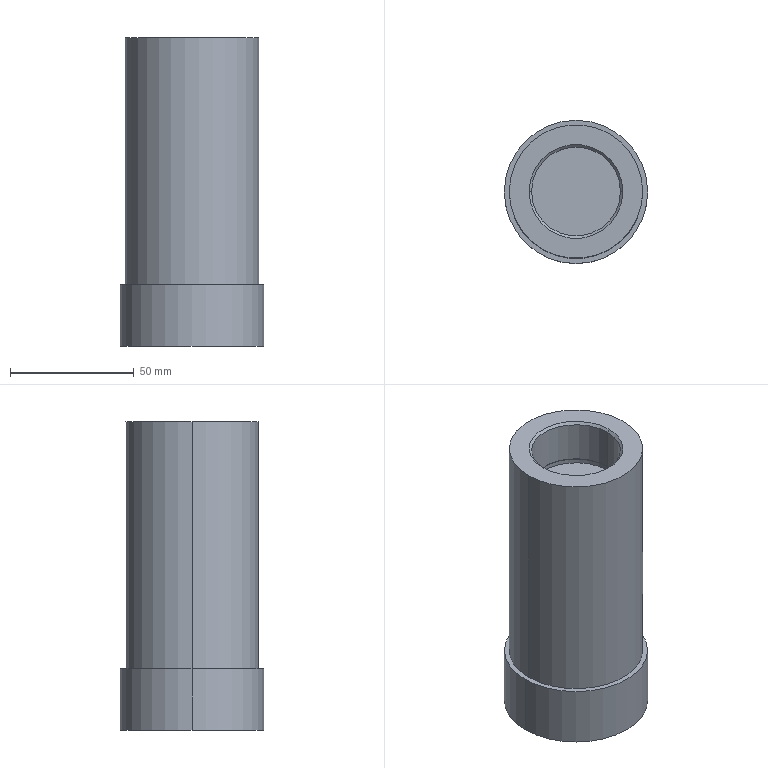Part | SolidWorks | features ICE 5, Chamfer 2, Extrusion 1 | 1 solid | 23 faces | box 58 x 58 x 125 mm | volume 229241 mm3 | cylinder 12 | plane 7 | cone 4 | commonest cylinder face diameters 36 x2 36.5 x2 48 x2 48.2 x2 54 x2 58 x2
STEP:
#1=CARTESIAN_POINT('',(-18.,0.,124.));
#2=VERTEX_POINT('',#1);
#3=CARTESIAN_POINT('',(18.,0.,124.));
#4=VERTEX_POINT('',#3);
#5=CARTESIAN_POINT('',(0.,0.,124.));
#6=DIRECTION('',(0.,0.,1.));
#7=DIRECTION('',(1.,0.,0.));
#8=AXIS2_PLACEMENT_3D('',#5,#6,#7);
#9=CIRCLE('',#8,18.);
#10=EDGE_CURVE('',#2,#4,#9,.T.);
#11=ORIENTED_EDGE('',*,*,#10,.F.);
#12=CARTESIAN_POINT('',(-19.,0.,125.));
#13=VERTEX_POINT('',#12);
#14=CARTESIAN_POINT('',(-18.,0.,124.));
#15=DIRECTION('',(-0.7071,0.,0.7071));
#16=VECTOR('',#15,1000.);
#17=LINE('',#14,#16);
#18=EDGE_CURVE('',#2,#13,#17,.T.);
#19=ORIENTED_EDGE('',*,*,#18,.T.);
#20=CARTESIAN_POINT('',(19.,0.,125.));
#21=VERTEX_POINT('',#20);
#22=CARTESIAN_POINT('',(0.,0.,125.));
#23=DIRECTION('',(0.,0.,-1.));
#24=DIRECTION('',(1.,0.,0.));
#25=AXIS2_PLACEMENT_3D('',#22,#23,#24);
#26=CIRCLE('',#25,19.);
#27=EDGE_CURVE('',#21,#13,#26,.T.);
#28=ORIENTED_EDGE('',*,*,#27,.F.);
#29=CARTESIAN_POINT('',(18.,0.,124.));
#30=DIRECTION('',(0.7071,0.,0.7071));
#31=VECTOR('',#30,1000.);
#32=LINE('',#29,#31);
#33=EDGE_CURVE('',#4,#21,#32,.T.);
#34=ORIENTED_EDGE('',*,*,#33,.F.);
#35=EDGE_LOOP('',(#11,#19,#28,#34));
#36=FACE_OUTER_BOUND('',#35,.T.);
#37=CARTESIAN_POINT('',(0.,0.,124.));
#38=DIRECTION('',(0.,0.,1.));
#39=DIRECTION('',(1.,0.,0.));
#40=AXIS2_PLACEMENT_3D('',#37,#38,#39);
#41=CONICAL_SURFACE('',#40,18.,0.7854);
#42=ADVANCED_FACE('',(#36),#41,.F.);
#43=CARTESIAN_POINT('',(-18.25,0.,105.));
#44=VERTEX_POINT('',#43);
#45=CARTESIAN_POINT('',(18.25,0.,105.));
#46=VERTEX_POINT('',#45);
#47=CARTESIAN_POINT('',(0.,0.,105.));
#48=DIRECTION('',(0.,0.,1.));
#49=DIRECTION('',(1.,0.,0.));
#50=AXIS2_PLACEMENT_3D('',#47,#48,#49);
#51=CIRCLE('',#50,18.25);
#52=EDGE_CURVE('',#44,#46,#51,.T.);
#53=ORIENTED_EDGE('',*,*,#52,.F.);
#54=CARTESIAN_POINT('',(-18.25,0.,107.));
#55=VERTEX_POINT('',#54);
#56=CARTESIAN_POINT('',(-18.25,0.,105.));
#57=DIRECTION('',(0.,0.,1.));
#58=VECTOR('',#57,1000.);
#59=LINE('',#56,#58);
#60=EDGE_CURVE('',#44,#55,#59,.T.);
#61=ORIENTED_EDGE('',*,*,#60,.T.);
#62=CARTESIAN_POINT('',(18.25,0.,107.));
#63=VERTEX_POINT('',#62);
#64=CARTESIAN_POINT('',(0.,0.,107.));
#65=DIRECTION('',(0.,0.,1.));
#66=DIRECTION('',(1.,0.,0.));
#67=AXIS2_PLACEMENT_3D('',#64,#65,#66);
#68=CIRCLE('',#67,18.25);
#69=EDGE_CURVE('',#55,#63,#68,.T.);
#70=ORIENTED_EDGE('',*,*,#69,.T.);
#71=CARTESIAN_POINT('',(18.25,0.,105.));
#72=DIRECTION('',(0.,0.,1.));
#73=VECTOR('',#72,1000.);
#74=LINE('',#71,#73);
#75=EDGE_CURVE('',#46,#63,#74,.T.);
#76=ORIENTED_EDGE('',*,*,#75,.F.);
#77=EDGE_LOOP('',(#53,#61,#70,#76));
#78=FACE_OUTER_BOUND('',#77,.T.);
#79=CARTESIAN_POINT('',(0.,0.,105.));
#80=DIRECTION('',(0.,0.,1.));
#81=DIRECTION('',(1.,0.,0.));
#82=AXIS2_PLACEMENT_3D('',#79,#80,#81);
#83=CYLINDRICAL_SURFACE('',#82,18.25);
#84=ADVANCED_FACE('',(#78),#83,.F.);
#85=CARTESIAN_POINT('',(-18.,0.,107.));
#86=VERTEX_POINT('',#85);
#87=CARTESIAN_POINT('',(18.,0.,107.));
#88=VERTEX_POINT('',#87);
#89=CARTESIAN_POINT('',(0.,0.,107.));
#90=DIRECTION('',(0.,0.,1.));
#91=DIRECTION('',(1.,0.,0.));
#92=AXIS2_PLACEMENT_3D('',#89,#90,#91);
#93=CIRCLE('',#92,18.);
#94=EDGE_CURVE('',#86,#88,#93,.T.);
#95=ORIENTED_EDGE('',*,*,#94,.F.);
#96=CARTESIAN_POINT('',(-18.,0.,107.));
#97=DIRECTION('',(0.,0.,1.));
#98=VECTOR('',#97,1000.);
#99=LINE('',#96,#98);
#100=EDGE_CURVE('',#86,#2,#99,.T.);
#101=ORIENTED_EDGE('',*,*,#100,.T.);
#102=ORIENTED_EDGE('',*,*,#10,.T.);
#103=CARTESIAN_POINT('',(18.,0.,107.));
#104=DIRECTION('',(0.,0.,1.));
#105=VECTOR('',#104,1000.);
#106=LINE('',#103,#105);
#107=EDGE_CURVE('',#88,#4,#106,.T.);
#108=ORIENTED_EDGE('',*,*,#107,.F.);
#109=EDGE_LOOP('',(#95,#101,#102,#108));
#110=FACE_OUTER_BOUND('',#109,.T.);
#111=CARTESIAN_POINT('',(0.,0.,107.));
#112=DIRECTION('',(0.,0.,1.));
#113=DIRECTION('',(1.,0.,0.));
#114=AXIS2_PLACEMENT_3D('',#111,#112,#113);
#115=CYLINDRICAL_SURFACE('',#114,18.);
#116=ADVANCED_FACE('',(#110),#115,.F.);
#117=CARTESIAN_POINT('',(24.,0.,1.));
#118=VERTEX_POINT('',#117);
#119=CARTESIAN_POINT('',(-24.,0.,1.));
#120=VERTEX_POINT('',#119);
#121=CARTESIAN_POINT('',(0.,0.,1.));
#122=DIRECTION('',(0.,0.,-1.));
#123=DIRECTION('',(1.,0.,0.));
#124=AXIS2_PLACEMENT_3D('',#121,#122,#123);
#125=CIRCLE('',#124,24.);
#126=EDGE_CURVE('',#118,#120,#125,.T.);
#127=ORIENTED_EDGE('',*,*,#126,.F.);
#128=CARTESIAN_POINT('',(25.,0.,0.));
#129=VERTEX_POINT('',#128);
#130=CARTESIAN_POINT('',(24.,0.,1.));
#131=DIRECTION('',(0.7071,0.,-0.7071));
#132=VECTOR('',#131,1000.);
#133=LINE('',#130,#132);
#134=EDGE_CURVE('',#118,#129,#133,.T.);
#135=ORIENTED_EDGE('',*,*,#134,.T.);
#136=CARTESIAN_POINT('',(-25.,0.,0.));
#137=VERTEX_POINT('',#136);
#138=CARTESIAN_POINT('',(0.,0.,0.));
#139=DIRECTION('',(0.,0.,1.));
#140=DIRECTION('',(1.,0.,0.));
#141=AXIS2_PLACEMENT_3D('',#138,#139,#140);
#142=CIRCLE('',#141,25.);
#143=EDGE_CURVE('',#137,#129,#142,.T.);
#144=ORIENTED_EDGE('',*,*,#143,.F.);
#145=CARTESIAN_POINT('',(-24.,0.,1.));
#146=DIRECTION('',(-0.7071,0.,-0.7071));
#147=VECTOR('',#146,1000.);
#148=LINE('',#145,#147);
#149=EDGE_CURVE('',#120,#137,#148,.T.);
#150=ORIENTED_EDGE('',*,*,#149,.F.);
#151=EDGE_LOOP('',(#127,#135,#144,#150));
#152=FACE_OUTER_BOUND('',#151,.T.);
#153=CARTESIAN_POINT('',(0.,0.,1.));
#154=DIRECTION('',(0.,0.,-1.));
#155=DIRECTION('',(-1.,0.,0.));
#156=AXIS2_PLACEMENT_3D('',#153,#154,#155);
#157=CONICAL_SURFACE('',#156,24.,0.7854);
#158=ADVANCED_FACE('',(#152),#157,.F.);
#159=CARTESIAN_POINT('',(24.1,0.,25.));
#160=VERTEX_POINT('',#159);
#161=CARTESIAN_POINT('',(-24.1,0.,25.));
#162=VERTEX_POINT('',#161);
#163=CARTESIAN_POINT('',(0.,0.,25.));
#164=DIRECTION('',(0.,0.,-1.));
#165=DIRECTION('',(-1.,0.,0.));
#166=AXIS2_PLACEMENT_3D('',#163,#164,#165);
#167=CIRCLE('',#166,24.1);
#168=EDGE_CURVE('',#160,#162,#167,.T.);
#169=ORIENTED_EDGE('',*,*,#168,.F.);
#170=CARTESIAN_POINT('',(24.1,0.,22.));
#171=VERTEX_POINT('',#170);
#172=CARTESIAN_POINT('',(24.1,0.,25.));
#173=DIRECTION('',(0.,0.,-1.));
#174=VECTOR('',#173,1000.);
#175=LINE('',#172,#174);
#176=EDGE_CURVE('',#160,#171,#175,.T.);
#177=ORIENTED_EDGE('',*,*,#176,.T.);
#178=CARTESIAN_POINT('',(-24.1,0.,22.));
#179=VERTEX_POINT('',#178);
#180=CARTESIAN_POINT('',(0.,0.,22.));
#181=DIRECTION('',(0.,0.,-1.));
#182=DIRECTION('',(-1.,0.,0.));
#183=AXIS2_PLACEMENT_3D('',#180,#181,#182);
#184=CIRCLE('',#183,24.1);
#185=EDGE_CURVE('',#171,#179,#184,.T.);
#186=ORIENTED_EDGE('',*,*,#185,.T.);
#187=CARTESIAN_POINT('',(-24.1,0.,25.));
#188=DIRECTION('',(0.,0.,-1.));
#189=VECTOR('',#188,1000.);
#190=LINE('',#187,#189);
#191=EDGE_CURVE('',#162,#179,#190,.T.);
#192=ORIENTED_EDGE('',*,*,#191,.F.);
#193=EDGE_LOOP('',(#169,#177,#186,#192));
#194=FACE_OUTER_BOUND('',#193,.T.);
#195=CARTESIAN_POINT('',(0.,0.,25.));
#196=DIRECTION('',(0.,0.,-1.));
#197=DIRECTION('',(-1.,0.,0.));
#198=AXIS2_PLACEMENT_3D('',#195,#196,#197);
#199=CYLINDRICAL_SURFACE('',#198,24.1);
#200=ADVANCED_FACE('',(#194),#199,.F.);
#201=CARTESIAN_POINT('',(24.,0.,22.));
#202=VERTEX_POINT('',#201);
#203=CARTESIAN_POINT('',(-24.,0.,22.));
#204=VERTEX_POINT('',#203);
#205=CARTESIAN_POINT('',(0.,0.,22.));
#206=DIRECTION('',(0.,0.,-1.));
#207=DIRECTION('',(-1.,0.,0.));
#208=AXIS2_PLACEMENT_3D('',#205,#206,#207);
#209=CIRCLE('',#208,24.);
#210=EDGE_CURVE('',#202,#204,#209,.T.);
#211=ORIENTED_EDGE('',*,*,#210,.F.);
#212=CARTESIAN_POINT('',(24.,0.,22.));
#213=DIRECTION('',(0.,0.,-1.));
#214=VECTOR('',#213,1000.);
#215=LINE('',#212,#214);
#216=EDGE_CURVE('',#202,#118,#215,.T.);
#217=ORIENTED_EDGE('',*,*,#216,.T.);
#218=ORIENTED_EDGE('',*,*,#126,.T.);
#219=CARTESIAN_POINT('',(-24.,0.,22.));
#220=DIRECTION('',(0.,0.,-1.));
#221=VECTOR('',#220,1000.);
#222=LINE('',#219,#221);
#223=EDGE_CURVE('',#204,#120,#222,.T.);
#224=ORIENTED_EDGE('',*,*,#223,.F.);
#225=EDGE_LOOP('',(#211,#217,#218,#224));
#226=FACE_OUTER_BOUND('',#225,.T.);
#227=CARTESIAN_POINT('',(0.,0.,22.));
#228=DIRECTION('',(0.,0.,-1.));
#229=DIRECTION('',(-1.,0.,0.));
#230=AXIS2_PLACEMENT_3D('',#227,#228,#229);
#231=CYLINDRICAL_SURFACE('',#230,24.);
#232=ADVANCED_FACE('',(#226),#231,.F.);
#233=CARTESIAN_POINT('',(27.,0.,125.));
#234=VERTEX_POINT('',#233);
#235=CARTESIAN_POINT('',(-27.,0.,125.));
#236=VERTEX_POINT('',#235);
#237=CARTESIAN_POINT('',(0.,0.,125.));
#238=DIRECTION('',(0.,0.,1.));
#239=DIRECTION('',(1.,0.,0.));
#240=AXIS2_PLACEMENT_3D('',#237,#238,#239);
#241=CIRCLE('',#240,27.);
#242=EDGE_CURVE('',#234,#236,#241,.T.);
#243=ORIENTED_EDGE('',*,*,#242,.F.);
#244=CARTESIAN_POINT('',(27.,0.,25.));
#245=VERTEX_POINT('',#244);
#246=CARTESIAN_POINT('',(27.,0.,125.));
#247=DIRECTION('',(0.,0.,-1.));
#248=VECTOR('',#247,1000.);
#249=LINE('',#246,#248);
#250=EDGE_CURVE('',#234,#245,#249,.T.);
#251=ORIENTED_EDGE('',*,*,#250,.T.);
#252=CARTESIAN_POINT('',(-27.,0.,25.));
#253=VERTEX_POINT('',#252);
#254=CARTESIAN_POINT('',(0.,0.,25.));
#255=DIRECTION('',(0.,0.,1.));
#256=DIRECTION('',(1.,0.,0.));
#257=AXIS2_PLACEMENT_3D('',#254,#255,#256);
#258=CIRCLE('',#257,27.);
#259=EDGE_CURVE('',#245,#253,#258,.T.);
#260=ORIENTED_EDGE('',*,*,#259,.T.);
#261=CARTESIAN_POINT('',(-27.,0.,125.));
#262=DIRECTION('',(0.,0.,-1.));
#263=VECTOR('',#262,1000.);
#264=LINE('',#261,#263);
#265=EDGE_CURVE('',#236,#253,#264,.T.);
#266=ORIENTED_EDGE('',*,*,#265,.F.);
#267=EDGE_LOOP('',(#243,#251,#260,#266));
#268=FACE_OUTER_BOUND('',#267,.T.);
#269=CARTESIAN_POINT('',(0.,0.,125.));
#270=DIRECTION('',(0.,0.,-1.));
#271=DIRECTION('',(-1.,0.,0.));
#272=AXIS2_PLACEMENT_3D('',#269,#270,#271);
#273=CYLINDRICAL_SURFACE('',#272,27.);
#274=ADVANCED_FACE('',(#268),#273,.T.);
#275=CARTESIAN_POINT('',(29.,0.,25.));
#276=VERTEX_POINT('',#275);
#277=CARTESIAN_POINT('',(-29.,0.,25.));
#278=VERTEX_POINT('',#277);
#279=CARTESIAN_POINT('',(0.,0.,25.));
#280=DIRECTION('',(0.,0.,1.));
#281=DIRECTION('',(1.,0.,0.));
#282=AXIS2_PLACEMENT_3D('',#279,#280,#281);
#283=CIRCLE('',#282,29.);
#284=EDGE_CURVE('',#276,#278,#283,.T.);
#285=ORIENTED_EDGE('',*,*,#284,.F.);
#286=CARTESIAN_POINT('',(29.,0.,0.));
#287=VERTEX_POINT('',#286);
#288=CARTESIAN_POINT('',(29.,0.,25.));
#289=DIRECTION('',(0.,0.,-1.));
#290=VECTOR('',#289,1000.);
#291=LINE('',#288,#290);
#292=EDGE_CURVE('',#276,#287,#291,.T.);
#293=ORIENTED_EDGE('',*,*,#292,.T.);
#294=CARTESIAN_POINT('',(-29.,0.,0.));
#295=VERTEX_POINT('',#294);
#296=CARTESIAN_POINT('',(0.,0.,0.));
#297=DIRECTION('',(0.,0.,1.));
#298=DIRECTION('',(1.,0.,0.));
#299=AXIS2_PLACEMENT_3D('',#296,#297,#298);
#300=CIRCLE('',#299,29.);
#301=EDGE_CURVE('',#287,#295,#300,.T.);
#302=ORIENTED_EDGE('',*,*,#301,.T.);
#303=CARTESIAN_POINT('',(-29.,0.,25.));
#304=DIRECTION('',(0.,0.,-1.));
#305=VECTOR('',#304,1000.);
#306=LINE('',#303,#305);
#307=EDGE_CURVE('',#278,#295,#306,.T.);
#308=ORIENTED_EDGE('',*,*,#307,.F.);
#309=EDGE_LOOP('',(#285,#293,#302,#308));
#310=FACE_OUTER_BOUND('',#309,.T.);
#311=CARTESIAN_POINT('',(0.,0.,25.));
#312=DIRECTION('',(0.,0.,-1.));
#313=DIRECTION('',(-1.,0.,0.));
#314=AXIS2_PLACEMENT_3D('',#311,#312,#313);
#315=CYLINDRICAL_SURFACE('',#314,29.);
#316=ADVANCED_FACE('',(#310),#315,.T.);
#317=ORIENTED_EDGE('',*,*,#292,.F.);
#318=CARTESIAN_POINT('',(0.,0.,25.));
#319=DIRECTION('',(0.,0.,1.));
#320=DIRECTION('',(1.,0.,0.));
#321=AXIS2_PLACEMENT_3D('',#318,#319,#320);
#322=CIRCLE('',#321,29.);
#323=EDGE_CURVE('',#278,#276,#322,.T.);
#324=ORIENTED_EDGE('',*,*,#323,.F.);
#325=ORIENTED_EDGE('',*,*,#307,.T.);
#326=CARTESIAN_POINT('',(0.,0.,0.));
#327=DIRECTION('',(0.,0.,1.));
#328=DIRECTION('',(1.,0.,0.));
#329=AXIS2_PLACEMENT_3D('',#326,#327,#328);
#330=CIRCLE('',#329,29.);
#331=EDGE_CURVE('',#295,#287,#330,.T.);
#332=ORIENTED_EDGE('',*,*,#331,.T.);
#333=EDGE_LOOP('',(#317,#324,#325,#332));
#334=FACE_OUTER_BOUND('',#333,.T.);
#335=CARTESIAN_POINT('',(0.,0.,25.));
#336=DIRECTION('',(0.,0.,-1.));
#337=DIRECTION('',(-1.,0.,0.));
#338=AXIS2_PLACEMENT_3D('',#335,#336,#337);
#339=CYLINDRICAL_SURFACE('',#338,29.);
#340=ADVANCED_FACE('',(#334),#339,.T.);
#341=CARTESIAN_POINT('',(0.,0.,25.));
#342=DIRECTION('',(0.,0.,1.));
#343=DIRECTION('',(1.,0.,0.));
#344=AXIS2_PLACEMENT_3D('',#341,#342,#343);
#345=CIRCLE('',#344,27.);
#346=EDGE_CURVE('',#253,#245,#345,.T.);
#347=ORIENTED_EDGE('',*,*,#346,.F.);
#348=ORIENTED_EDGE('',*,*,#259,.F.);
#349=EDGE_LOOP('',(#347,#348));
#350=FACE_BOUND('',#349,.T.);
#351=ORIENTED_EDGE('',*,*,#323,.T.);
#352=ORIENTED_EDGE('',*,*,#284,.T.);
#353=EDGE_LOOP('',(#351,#352));
#354=FACE_OUTER_BOUND('',#353,.T.);
#355=CARTESIAN_POINT('',(0.,0.,25.));
#356=DIRECTION('',(0.,0.,1.));
#357=DIRECTION('',(1.,0.,0.));
#358=AXIS2_PLACEMENT_3D('',#355,#356,#357);
#359=PLANE('',#358);
#360=ADVANCED_FACE('',(#350,#354),#359,.T.);
#361=ORIENTED_EDGE('',*,*,#143,.T.);
#362=CARTESIAN_POINT('',(0.,0.,0.));
#363=DIRECTION('',(0.,0.,1.));
#364=DIRECTION('',(1.,0.,0.));
#365=AXIS2_PLACEMENT_3D('',#362,#363,#364);
#366=CIRCLE('',#365,25.);
#367=EDGE_CURVE('',#129,#137,#366,.T.);
#368=ORIENTED_EDGE('',*,*,#367,.T.);
#369=EDGE_LOOP('',(#361,#368));
#370=FACE_BOUND('',#369,.T.);
#371=ORIENTED_EDGE('',*,*,#331,.F.);
#372=ORIENTED_EDGE('',*,*,#301,.F.);
#373=EDGE_LOOP('',(#371,#372));
#374=FACE_OUTER_BOUND('',#373,.T.);
#375=CARTESIAN_POINT('',(0.,0.,0.));
#376=DIRECTION('',(0.,0.,1.));
#377=DIRECTION('',(1.,0.,0.));
#378=AXIS2_PLACEMENT_3D('',#375,#376,#377);
#379=PLANE('',#378);
#380=ADVANCED_FACE('',(#370,#374),#379,.F.);
#381=ORIENTED_EDGE('',*,*,#250,.F.);
#382=CARTESIAN_POINT('',(0.,0.,125.));
#383=DIRECTION('',(0.,0.,1.));
#384=DIRECTION('',(1.,0.,0.));
#385=AXIS2_PLACEMENT_3D('',#382,#383,#384);
#386=CIRCLE('',#385,27.);
#387=EDGE_CURVE('',#236,#234,#386,.T.);
#388=ORIENTED_EDGE('',*,*,#387,.F.);
#389=ORIENTED_EDGE('',*,*,#265,.T.);
#390=ORIENTED_EDGE('',*,*,#346,.T.);
#391=EDGE_LOOP('',(#381,#388,#389,#390));
#392=FACE_OUTER_BOUND('',#391,.T.);
#393=CARTESIAN_POINT('',(0.,0.,125.));
#394=DIRECTION('',(0.,0.,-1.));
#395=DIRECTION('',(-1.,0.,0.));
#396=AXIS2_PLACEMENT_3D('',#393,#394,#395);
#397=CYLINDRICAL_SURFACE('',#396,27.);
#398=ADVANCED_FACE('',(#392),#397,.T.);
#399=ORIENTED_EDGE('',*,*,#27,.T.);
#400=CARTESIAN_POINT('',(0.,0.,125.));
#401=DIRECTION('',(0.,0.,-1.));
#402=DIRECTION('',(1.,0.,0.));
#403=AXIS2_PLACEMENT_3D('',#400,#401,#402);
#404=CIRCLE('',#403,19.);
#405=EDGE_CURVE('',#13,#21,#404,.T.);
#406=ORIENTED_EDGE('',*,*,#405,.T.);
#407=EDGE_LOOP('',(#399,#406));
#408=FACE_BOUND('',#407,.T.);
#409=ORIENTED_EDGE('',*,*,#387,.T.);
#410=ORIENTED_EDGE('',*,*,#242,.T.);
#411=EDGE_LOOP('',(#409,#410));
#412=FACE_OUTER_BOUND('',#411,.T.);
#413=CARTESIAN_POINT('',(0.,0.,125.));
#414=DIRECTION('',(0.,0.,1.));
#415=DIRECTION('',(1.,0.,0.));
#416=AXIS2_PLACEMENT_3D('',#413,#414,#415);
#417=PLANE('',#416);
#418=ADVANCED_FACE('',(#408,#412),#417,.T.);
#419=ORIENTED_EDGE('',*,*,#216,.F.);
#420=CARTESIAN_POINT('',(0.,0.,22.));
#421=DIRECTION('',(0.,0.,-1.));
#422=DIRECTION('',(-1.,0.,0.));
#423=AXIS2_PLACEMENT_3D('',#420,#421,#422);
#424=CIRCLE('',#423,24.);
#425=EDGE_CURVE('',#204,#202,#424,.T.);
#426=ORIENTED_EDGE('',*,*,#425,.F.);
#427=ORIENTED_EDGE('',*,*,#223,.T.);
#428=CARTESIAN_POINT('',(0.,0.,1.));
#429=DIRECTION('',(0.,0.,-1.));
#430=DIRECTION('',(1.,0.,0.));
#431=AXIS2_PLACEMENT_3D('',#428,#429,#430);
#432=CIRCLE('',#431,24.);
#433=EDGE_CURVE('',#120,#118,#432,.T.);
#434=ORIENTED_EDGE('',*,*,#433,.T.);
#435=EDGE_LOOP('',(#419,#426,#427,#434));
#436=FACE_OUTER_BOUND('',#435,.T.);
#437=CARTESIAN_POINT('',(0.,0.,22.));
#438=DIRECTION('',(0.,0.,-1.));
#439=DIRECTION('',(-1.,0.,0.));
#440=AXIS2_PLACEMENT_3D('',#437,#438,#439);
#441=CYLINDRICAL_SURFACE('',#440,24.);
#442=ADVANCED_FACE('',(#436),#441,.F.);
#443=ORIENTED_EDGE('',*,*,#176,.F.);
#444=CARTESIAN_POINT('',(0.,0.,25.));
#445=DIRECTION('',(0.,0.,-1.));
#446=DIRECTION('',(-1.,0.,0.));
#447=AXIS2_PLACEMENT_3D('',#444,#445,#446);
#448=CIRCLE('',#447,24.1);
#449=EDGE_CURVE('',#162,#160,#448,.T.);
#450=ORIENTED_EDGE('',*,*,#449,.F.);
#451=ORIENTED_EDGE('',*,*,#191,.T.);
#452=CARTESIAN_POINT('',(0.,0.,22.));
#453=DIRECTION('',(0.,0.,-1.));
#454=DIRECTION('',(-1.,0.,0.));
#455=AXIS2_PLACEMENT_3D('',#452,#453,#454);
#456=CIRCLE('',#455,24.1);
#457=EDGE_CURVE('',#179,#171,#456,.T.);
#458=ORIENTED_EDGE('',*,*,#457,.T.);
#459=EDGE_LOOP('',(#443,#450,#451,#458));
#460=FACE_OUTER_BOUND('',#459,.T.);
#461=CARTESIAN_POINT('',(0.,0.,25.));
#462=DIRECTION('',(0.,0.,-1.));
#463=DIRECTION('',(-1.,0.,0.));
#464=AXIS2_PLACEMENT_3D('',#461,#462,#463);
#465=CYLINDRICAL_SURFACE('',#464,24.1);
#466=ADVANCED_FACE('',(#460),#465,.F.);
#467=ORIENTED_EDGE('',*,*,#449,.T.);
#468=ORIENTED_EDGE('',*,*,#168,.T.);
#469=EDGE_LOOP('',(#467,#468));
#470=FACE_OUTER_BOUND('',#469,.T.);
#471=CARTESIAN_POINT('',(0.,0.,25.));
#472=DIRECTION('',(0.,0.,-1.));
#473=DIRECTION('',(-1.,0.,0.));
#474=AXIS2_PLACEMENT_3D('',#471,#472,#473);
#475=PLANE('',#474);
#476=ADVANCED_FACE('',(#470),#475,.T.);
#477=ORIENTED_EDGE('',*,*,#425,.T.);
#478=ORIENTED_EDGE('',*,*,#210,.T.);
#479=EDGE_LOOP('',(#477,#478));
#480=FACE_BOUND('',#479,.T.);
#481=ORIENTED_EDGE('',*,*,#457,.F.);
#482=ORIENTED_EDGE('',*,*,#185,.F.);
#483=EDGE_LOOP('',(#481,#482));
#484=FACE_OUTER_BOUND('',#483,.T.);
#485=CARTESIAN_POINT('',(0.,0.,22.));
#486=DIRECTION('',(0.,0.,-1.));
#487=DIRECTION('',(-1.,0.,0.));
#488=AXIS2_PLACEMENT_3D('',#485,#486,#487);
#489=PLANE('',#488);
#490=ADVANCED_FACE('',(#480,#484),#489,.F.);
#491=ORIENTED_EDGE('',*,*,#134,.F.);
#492=ORIENTED_EDGE('',*,*,#433,.F.);
#493=ORIENTED_EDGE('',*,*,#149,.T.);
#494=ORIENTED_EDGE('',*,*,#367,.F.);
#495=EDGE_LOOP('',(#491,#492,#493,#494));
#496=FACE_OUTER_BOUND('',#495,.T.);
#497=CARTESIAN_POINT('',(0.,0.,1.));
#498=DIRECTION('',(0.,0.,-1.));
#499=DIRECTION('',(-1.,0.,0.));
#500=AXIS2_PLACEMENT_3D('',#497,#498,#499);
#501=CONICAL_SURFACE('',#500,24.,0.7854);
#502=ADVANCED_FACE('',(#496),#501,.F.);
#503=ORIENTED_EDGE('',*,*,#100,.F.);
#504=CARTESIAN_POINT('',(0.,0.,107.));
#505=DIRECTION('',(0.,0.,1.));
#506=DIRECTION('',(1.,0.,0.));
#507=AXIS2_PLACEMENT_3D('',#504,#505,#506);
#508=CIRCLE('',#507,18.);
#509=EDGE_CURVE('',#88,#86,#508,.T.);
#510=ORIENTED_EDGE('',*,*,#509,.F.);
#511=ORIENTED_EDGE('',*,*,#107,.T.);
#512=CARTESIAN_POINT('',(0.,0.,124.));
#513=DIRECTION('',(0.,0.,1.));
#514=DIRECTION('',(1.,0.,0.));
#515=AXIS2_PLACEMENT_3D('',#512,#513,#514);
#516=CIRCLE('',#515,18.);
#517=EDGE_CURVE('',#4,#2,#516,.T.);
#518=ORIENTED_EDGE('',*,*,#517,.T.);
#519=EDGE_LOOP('',(#503,#510,#511,#518));
#520=FACE_OUTER_BOUND('',#519,.T.);
#521=CARTESIAN_POINT('',(0.,0.,107.));
#522=DIRECTION('',(0.,0.,1.));
#523=DIRECTION('',(1.,0.,0.));
#524=AXIS2_PLACEMENT_3D('',#521,#522,#523);
#525=CYLINDRICAL_SURFACE('',#524,18.);
#526=ADVANCED_FACE('',(#520),#525,.F.);
#527=ORIENTED_EDGE('',*,*,#60,.F.);
#528=CARTESIAN_POINT('',(0.,0.,105.));
#529=DIRECTION('',(0.,0.,1.));
#530=DIRECTION('',(1.,0.,0.));
#531=AXIS2_PLACEMENT_3D('',#528,#529,#530);
#532=CIRCLE('',#531,18.25);
#533=EDGE_CURVE('',#46,#44,#532,.T.);
#534=ORIENTED_EDGE('',*,*,#533,.F.);
#535=ORIENTED_EDGE('',*,*,#75,.T.);
#536=CARTESIAN_POINT('',(0.,0.,107.));
#537=DIRECTION('',(0.,0.,1.));
#538=DIRECTION('',(1.,0.,0.));
#539=AXIS2_PLACEMENT_3D('',#536,#537,#538);
#540=CIRCLE('',#539,18.25);
#541=EDGE_CURVE('',#63,#55,#540,.T.);
#542=ORIENTED_EDGE('',*,*,#541,.T.);
#543=EDGE_LOOP('',(#527,#534,#535,#542));
#544=FACE_OUTER_BOUND('',#543,.T.);
#545=CARTESIAN_POINT('',(0.,0.,105.));
#546=DIRECTION('',(0.,0.,1.));
#547=DIRECTION('',(1.,0.,0.));
#548=AXIS2_PLACEMENT_3D('',#545,#546,#547);
#549=CYLINDRICAL_SURFACE('',#548,18.25);
#550=ADVANCED_FACE('',(#544),#549,.F.);
#551=ORIENTED_EDGE('',*,*,#533,.T.);
#552=ORIENTED_EDGE('',*,*,#52,.T.);
#553=EDGE_LOOP('',(#551,#552));
#554=FACE_OUTER_BOUND('',#553,.T.);
#555=CARTESIAN_POINT('',(0.,0.,105.));
#556=DIRECTION('',(0.,0.,1.));
#557=DIRECTION('',(1.,0.,0.));
#558=AXIS2_PLACEMENT_3D('',#555,#556,#557);
#559=PLANE('',#558);
#560=ADVANCED_FACE('',(#554),#559,.T.);
#561=ORIENTED_EDGE('',*,*,#509,.T.);
#562=ORIENTED_EDGE('',*,*,#94,.T.);
#563=EDGE_LOOP('',(#561,#562));
#564=FACE_BOUND('',#563,.T.);
#565=ORIENTED_EDGE('',*,*,#541,.F.);
#566=ORIENTED_EDGE('',*,*,#69,.F.);
#567=EDGE_LOOP('',(#565,#566));
#568=FACE_OUTER_BOUND('',#567,.T.);
#569=CARTESIAN_POINT('',(0.,0.,107.));
#570=DIRECTION('',(0.,0.,1.));
#571=DIRECTION('',(1.,0.,0.));
#572=AXIS2_PLACEMENT_3D('',#569,#570,#571);
#573=PLANE('',#572);
#574=ADVANCED_FACE('',(#564,#568),#573,.F.);
#575=ORIENTED_EDGE('',*,*,#18,.F.);
#576=ORIENTED_EDGE('',*,*,#517,.F.);
#577=ORIENTED_EDGE('',*,*,#33,.T.);
#578=ORIENTED_EDGE('',*,*,#405,.F.);
#579=EDGE_LOOP('',(#575,#576,#577,#578));
#580=FACE_OUTER_BOUND('',#579,.T.);
#581=CARTESIAN_POINT('',(0.,0.,124.));
#582=DIRECTION('',(0.,0.,1.));
#583=DIRECTION('',(1.,0.,0.));
#584=AXIS2_PLACEMENT_3D('',#581,#582,#583);
#585=CONICAL_SURFACE('',#584,18.,0.7854);
#586=ADVANCED_FACE('',(#580),#585,.F.);
#587=CLOSED_SHELL('',(#42,#84,#116,#158,#200,#232,#274,#316,#340,#360,#380,#398,#418,#442,#466,#476,#490,#502,#526,#550,#560,#574,#586));
#588=MANIFOLD_SOLID_BREP('',#587);
#589=CARTESIAN_POINT('',(0.,0.,0.));
#590=DIRECTION('',(0.,0.,1.));
#591=DIRECTION('',(1.,0.,0.));
#592=AXIS2_PLACEMENT_3D('',#589,#590,#591);
#593=(LENGTH_UNIT()NAMED_UNIT(*)SI_UNIT(.MILLI.,.METRE.));
#594=UNCERTAINTY_MEASURE_WITH_UNIT(LENGTH_MEASURE(0.00001),#593,'','');
#595=(NAMED_UNIT(*)PLANE_ANGLE_UNIT()SI_UNIT($,.RADIAN.));
#596=(NAMED_UNIT(*)SI_UNIT($,.STERADIAN.)SOLID_ANGLE_UNIT());
#597=(GEOMETRIC_REPRESENTATION_CONTEXT(3)GLOBAL_UNCERTAINTY_ASSIGNED_CONTEXT((#594))GLOBAL_UNIT_ASSIGNED_CONTEXT((#593,#595,#596))REPRESENTATION_CONTEXT('',''));
#598=ADVANCED_BREP_SHAPE_REPRESENTATION('',(#588,#592),#597);